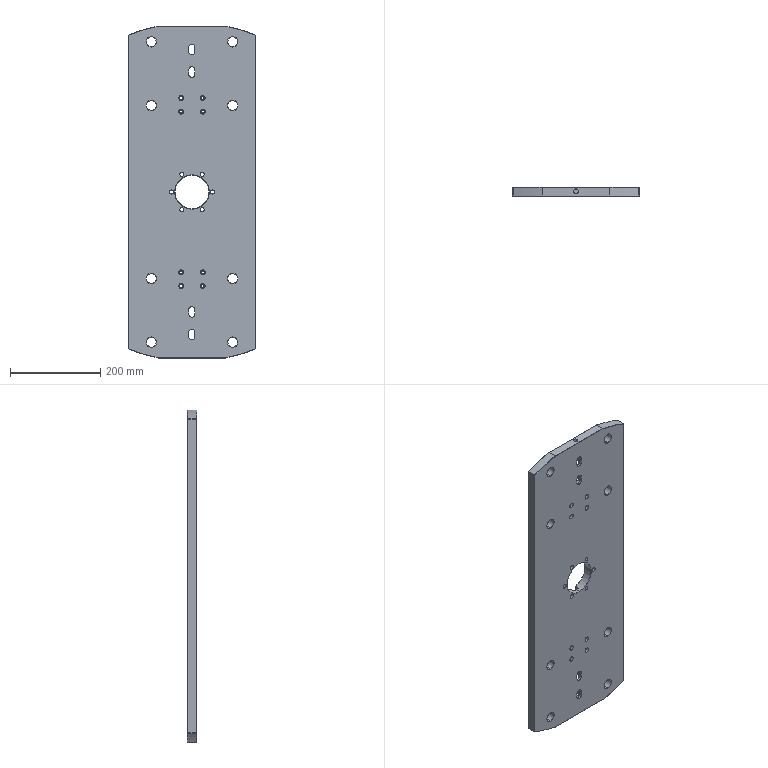Part | SolidWorks | features HoleWzd 5, MirrorPattern 5, Cut 4, ICE 3, Chamfer 1, Extrusion 1 | 1 solid | 204 faces | box 280 x 20 x 735 mm | volume 3763100 mm3 | cylinder 100 | plane 60 | cone 44 | commonest cylinder face diameters 3 x18 6.6 x16 11 x16 22 x16 9 x12 13.5 x12